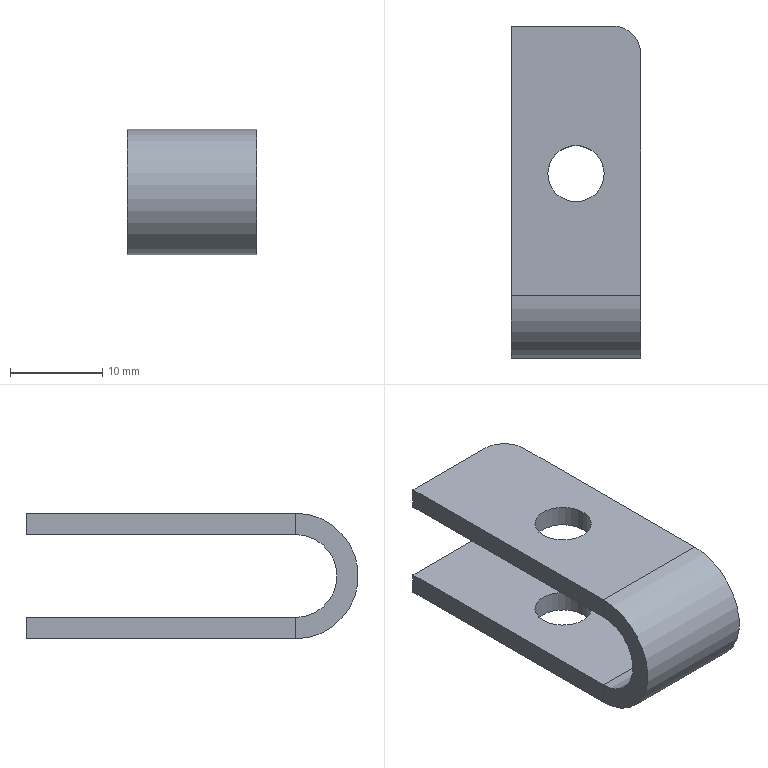Part | SolidWorks | features Fillet 1, FlatPattern 1, ICE 1, SMBaseFlange 1, SheetMetal 1 | 1 solid | 20 faces | box 14 x 36 x 13.6 mm | volume 2309 mm3 | plane 12 | cylinder 8 | commonest cylinder face diameters 6.1 x4 6 x2 9 x1 13.6 x1
STEP:
#1=CARTESIAN_POINT('',(3.95,13.2,4.5));
#2=VERTEX_POINT('',#1);
#3=CARTESIAN_POINT('',(10.05,13.2,4.5));
#4=VERTEX_POINT('',#3);
#5=CARTESIAN_POINT('',(7.,13.2,4.5));
#6=DIRECTION('',(0.,0.,1.));
#7=DIRECTION('',(0.,-1.,0.));
#8=AXIS2_PLACEMENT_3D('',#5,#6,#7);
#9=CIRCLE('',#8,3.05);
#10=EDGE_CURVE('',#2,#4,#9,.T.);
#11=ORIENTED_EDGE('',*,*,#10,.F.);
#12=CARTESIAN_POINT('',(3.95,13.2,6.8));
#13=VERTEX_POINT('',#12);
#14=CARTESIAN_POINT('',(3.95,13.2,-6.8));
#15=DIRECTION('',(0.,0.,1.));
#16=VECTOR('',#15,1000.);
#17=LINE('',#14,#16);
#18=EDGE_CURVE('',#2,#13,#17,.T.);
#19=ORIENTED_EDGE('',*,*,#18,.T.);
#20=CARTESIAN_POINT('',(10.05,13.2,6.8));
#21=VERTEX_POINT('',#20);
#22=CARTESIAN_POINT('',(7.,13.2,6.8));
#23=DIRECTION('',(0.,0.,1.));
#24=DIRECTION('',(1.,0.,0.));
#25=AXIS2_PLACEMENT_3D('',#22,#23,#24);
#26=CIRCLE('',#25,3.05);
#27=EDGE_CURVE('',#13,#21,#26,.T.);
#28=ORIENTED_EDGE('',*,*,#27,.T.);
#29=CARTESIAN_POINT('',(10.05,13.2,-6.8));
#30=DIRECTION('',(0.,0.,1.));
#31=VECTOR('',#30,1000.);
#32=LINE('',#29,#31);
#33=EDGE_CURVE('',#4,#21,#32,.T.);
#34=ORIENTED_EDGE('',*,*,#33,.F.);
#35=EDGE_LOOP('',(#11,#19,#28,#34));
#36=FACE_OUTER_BOUND('',#35,.T.);
#37=CARTESIAN_POINT('',(7.,13.2,-6.8));
#38=DIRECTION('',(0.,0.,1.));
#39=DIRECTION('',(1.,0.,0.));
#40=AXIS2_PLACEMENT_3D('',#37,#38,#39);
#41=CYLINDRICAL_SURFACE('',#40,3.05);
#42=ADVANCED_FACE('',(#36),#41,.F.);
#43=CARTESIAN_POINT('',(3.95,13.2,-6.8));
#44=VERTEX_POINT('',#43);
#45=CARTESIAN_POINT('',(10.05,13.2,-6.8));
#46=VERTEX_POINT('',#45);
#47=CARTESIAN_POINT('',(7.,13.2,-6.8));
#48=DIRECTION('',(0.,0.,1.));
#49=DIRECTION('',(1.,0.,0.));
#50=AXIS2_PLACEMENT_3D('',#47,#48,#49);
#51=CIRCLE('',#50,3.05);
#52=EDGE_CURVE('',#44,#46,#51,.T.);
#53=ORIENTED_EDGE('',*,*,#52,.F.);
#54=CARTESIAN_POINT('',(3.95,13.2,-4.5));
#55=VERTEX_POINT('',#54);
#56=CARTESIAN_POINT('',(3.95,13.2,-6.8));
#57=DIRECTION('',(0.,0.,1.));
#58=VECTOR('',#57,1000.);
#59=LINE('',#56,#58);
#60=EDGE_CURVE('',#44,#55,#59,.T.);
#61=ORIENTED_EDGE('',*,*,#60,.T.);
#62=CARTESIAN_POINT('',(10.05,13.2,-4.5));
#63=VERTEX_POINT('',#62);
#64=CARTESIAN_POINT('',(7.,13.2,-4.5));
#65=DIRECTION('',(0.,0.,-1.));
#66=DIRECTION('',(0.,1.,0.));
#67=AXIS2_PLACEMENT_3D('',#64,#65,#66);
#68=CIRCLE('',#67,3.05);
#69=EDGE_CURVE('',#63,#55,#68,.T.);
#70=ORIENTED_EDGE('',*,*,#69,.F.);
#71=CARTESIAN_POINT('',(10.05,13.2,-6.8));
#72=DIRECTION('',(0.,0.,1.));
#73=VECTOR('',#72,1000.);
#74=LINE('',#71,#73);
#75=EDGE_CURVE('',#46,#63,#74,.T.);
#76=ORIENTED_EDGE('',*,*,#75,.F.);
#77=EDGE_LOOP('',(#53,#61,#70,#76));
#78=FACE_OUTER_BOUND('',#77,.T.);
#79=CARTESIAN_POINT('',(7.,13.2,-6.8));
#80=DIRECTION('',(0.,0.,1.));
#81=DIRECTION('',(1.,0.,0.));
#82=AXIS2_PLACEMENT_3D('',#79,#80,#81);
#83=CYLINDRICAL_SURFACE('',#82,3.05);
#84=ADVANCED_FACE('',(#78),#83,.F.);
#85=CARTESIAN_POINT('',(14.,0.,6.8));
#86=VERTEX_POINT('',#85);
#87=CARTESIAN_POINT('',(14.,0.,4.5));
#88=VERTEX_POINT('',#87);
#89=CARTESIAN_POINT('',(14.,0.,6.8));
#90=DIRECTION('',(0.,0.,-1.));
#91=VECTOR('',#90,1000.);
#92=LINE('',#89,#91);
#93=EDGE_CURVE('',#86,#88,#92,.T.);
#94=ORIENTED_EDGE('',*,*,#93,.F.);
#95=CARTESIAN_POINT('',(14.,0.,-6.8));
#96=VERTEX_POINT('',#95);
#97=CARTESIAN_POINT('',(14.,0.,0.));
#98=DIRECTION('',(-1.,0.,0.));
#99=DIRECTION('',(0.,0.,-1.));
#100=AXIS2_PLACEMENT_3D('',#97,#98,#99);
#101=CIRCLE('',#100,6.8);
#102=EDGE_CURVE('',#96,#86,#101,.T.);
#103=ORIENTED_EDGE('',*,*,#102,.F.);
#104=CARTESIAN_POINT('',(14.,0.,-4.5));
#105=VERTEX_POINT('',#104);
#106=CARTESIAN_POINT('',(14.,0.,-4.5));
#107=DIRECTION('',(0.,0.,-1.));
#108=VECTOR('',#107,1000.);
#109=LINE('',#106,#108);
#110=EDGE_CURVE('',#105,#96,#109,.T.);
#111=ORIENTED_EDGE('',*,*,#110,.F.);
#112=CARTESIAN_POINT('',(14.,0.,0.));
#113=DIRECTION('',(-1.,0.,0.));
#114=DIRECTION('',(0.,0.,-1.));
#115=AXIS2_PLACEMENT_3D('',#112,#113,#114);
#116=CIRCLE('',#115,4.5);
#117=EDGE_CURVE('',#105,#88,#116,.T.);
#118=ORIENTED_EDGE('',*,*,#117,.T.);
#119=EDGE_LOOP('',(#94,#103,#111,#118));
#120=FACE_OUTER_BOUND('',#119,.T.);
#121=CARTESIAN_POINT('',(14.,0.,6.8));
#122=DIRECTION('',(1.,0.,0.));
#123=DIRECTION('',(0.,0.,-1.));
#124=AXIS2_PLACEMENT_3D('',#121,#122,#123);
#125=PLANE('',#124);
#126=ADVANCED_FACE('',(#120),#125,.T.);
#127=CARTESIAN_POINT('',(14.,26.2,4.5));
#128=VERTEX_POINT('',#127);
#129=CARTESIAN_POINT('',(14.,0.,4.5));
#130=DIRECTION('',(0.,1.,0.));
#131=VECTOR('',#130,1000.);
#132=LINE('',#129,#131);
#133=EDGE_CURVE('',#88,#128,#132,.T.);
#134=ORIENTED_EDGE('',*,*,#133,.T.);
#135=CARTESIAN_POINT('',(14.,26.2,6.8));
#136=VERTEX_POINT('',#135);
#137=CARTESIAN_POINT('',(14.,26.2,-4.5));
#138=DIRECTION('',(0.,0.,1.));
#139=VECTOR('',#138,1000.);
#140=LINE('',#137,#139);
#141=EDGE_CURVE('',#128,#136,#140,.T.);
#142=ORIENTED_EDGE('',*,*,#141,.T.);
#143=CARTESIAN_POINT('',(14.,0.,6.8));
#144=DIRECTION('',(0.,1.,0.));
#145=VECTOR('',#144,1000.);
#146=LINE('',#143,#145);
#147=EDGE_CURVE('',#86,#136,#146,.T.);
#148=ORIENTED_EDGE('',*,*,#147,.F.);
#149=ORIENTED_EDGE('',*,*,#93,.T.);
#150=EDGE_LOOP('',(#134,#142,#148,#149));
#151=FACE_OUTER_BOUND('',#150,.T.);
#152=CARTESIAN_POINT('',(14.,0.,-4.5));
#153=DIRECTION('',(1.,0.,0.));
#154=DIRECTION('',(0.,0.,-1.));
#155=AXIS2_PLACEMENT_3D('',#152,#153,#154);
#156=PLANE('',#155);
#157=ADVANCED_FACE('',(#151),#156,.T.);
#158=CARTESIAN_POINT('',(0.,0.,-6.8));
#159=VERTEX_POINT('',#158);
#160=CARTESIAN_POINT('',(0.,0.,-4.5));
#161=VERTEX_POINT('',#160);
#162=CARTESIAN_POINT('',(0.,0.,-6.8));
#163=DIRECTION('',(0.,0.,1.));
#164=VECTOR('',#163,1000.);
#165=LINE('',#162,#164);
#166=EDGE_CURVE('',#159,#161,#165,.T.);
#167=ORIENTED_EDGE('',*,*,#166,.F.);
#168=CARTESIAN_POINT('',(0.,0.,6.8));
#169=VERTEX_POINT('',#168);
#170=CARTESIAN_POINT('',(0.,0.,0.));
#171=DIRECTION('',(-1.,0.,0.));
#172=DIRECTION('',(0.,0.,-1.));
#173=AXIS2_PLACEMENT_3D('',#170,#171,#172);
#174=CIRCLE('',#173,6.8);
#175=EDGE_CURVE('',#159,#169,#174,.T.);
#176=ORIENTED_EDGE('',*,*,#175,.T.);
#177=CARTESIAN_POINT('',(0.,0.,4.5));
#178=VERTEX_POINT('',#177);
#179=CARTESIAN_POINT('',(0.,0.,4.5));
#180=DIRECTION('',(0.,0.,1.));
#181=VECTOR('',#180,1000.);
#182=LINE('',#179,#181);
#183=EDGE_CURVE('',#178,#169,#182,.T.);
#184=ORIENTED_EDGE('',*,*,#183,.F.);
#185=CARTESIAN_POINT('',(0.,0.,0.));
#186=DIRECTION('',(-1.,0.,0.));
#187=DIRECTION('',(0.,0.,-1.));
#188=AXIS2_PLACEMENT_3D('',#185,#186,#187);
#189=CIRCLE('',#188,4.5);
#190=EDGE_CURVE('',#161,#178,#189,.T.);
#191=ORIENTED_EDGE('',*,*,#190,.F.);
#192=EDGE_LOOP('',(#167,#176,#184,#191));
#193=FACE_OUTER_BOUND('',#192,.T.);
#194=CARTESIAN_POINT('',(0.,0.,-6.8));
#195=DIRECTION('',(-1.,0.,0.));
#196=DIRECTION('',(0.,0.,1.));
#197=AXIS2_PLACEMENT_3D('',#194,#195,#196);
#198=PLANE('',#197);
#199=ADVANCED_FACE('',(#193),#198,.T.);
#200=CARTESIAN_POINT('',(0.,29.2,-6.8));
#201=VERTEX_POINT('',#200);
#202=CARTESIAN_POINT('',(0.,29.2,-6.8));
#203=DIRECTION('',(0.,-1.,0.));
#204=VECTOR('',#203,1000.);
#205=LINE('',#202,#204);
#206=EDGE_CURVE('',#201,#159,#205,.T.);
#207=ORIENTED_EDGE('',*,*,#206,.T.);
#208=ORIENTED_EDGE('',*,*,#166,.T.);
#209=CARTESIAN_POINT('',(0.,29.2,-4.5));
#210=VERTEX_POINT('',#209);
#211=CARTESIAN_POINT('',(0.,29.2,-4.5));
#212=DIRECTION('',(0.,-1.,0.));
#213=VECTOR('',#212,1000.);
#214=LINE('',#211,#213);
#215=EDGE_CURVE('',#210,#161,#214,.T.);
#216=ORIENTED_EDGE('',*,*,#215,.F.);
#217=CARTESIAN_POINT('',(0.,29.2,-4.5));
#218=DIRECTION('',(0.,0.,-1.));
#219=VECTOR('',#218,1000.);
#220=LINE('',#217,#219);
#221=EDGE_CURVE('',#210,#201,#220,.T.);
#222=ORIENTED_EDGE('',*,*,#221,.T.);
#223=EDGE_LOOP('',(#207,#208,#216,#222));
#224=FACE_OUTER_BOUND('',#223,.T.);
#225=CARTESIAN_POINT('',(0.,0.,4.5));
#226=DIRECTION('',(-1.,0.,0.));
#227=DIRECTION('',(0.,0.,1.));
#228=AXIS2_PLACEMENT_3D('',#225,#226,#227);
#229=PLANE('',#228);
#230=ADVANCED_FACE('',(#224),#229,.T.);
#231=CARTESIAN_POINT('',(7.,13.2,4.5));
#232=DIRECTION('',(0.,0.,1.));
#233=DIRECTION('',(0.,-1.,0.));
#234=AXIS2_PLACEMENT_3D('',#231,#232,#233);
#235=CIRCLE('',#234,3.05);
#236=EDGE_CURVE('',#4,#2,#235,.T.);
#237=ORIENTED_EDGE('',*,*,#236,.T.);
#238=ORIENTED_EDGE('',*,*,#10,.T.);
#239=EDGE_LOOP('',(#237,#238));
#240=FACE_BOUND('',#239,.T.);
#241=CARTESIAN_POINT('',(11.,29.2,4.5));
#242=VERTEX_POINT('',#241);
#243=CARTESIAN_POINT('',(0.,29.2,4.5));
#244=VERTEX_POINT('',#243);
#245=CARTESIAN_POINT('',(14.,29.2,4.5));
#246=DIRECTION('',(-1.,0.,0.));
#247=VECTOR('',#246,1000.);
#248=LINE('',#245,#247);
#249=EDGE_CURVE('',#242,#244,#248,.T.);
#250=ORIENTED_EDGE('',*,*,#249,.F.);
#251=CARTESIAN_POINT('',(11.,26.2,4.5));
#252=DIRECTION('',(0.,0.,-1.));
#253=DIRECTION('',(0.,-1.,0.));
#254=AXIS2_PLACEMENT_3D('',#251,#252,#253);
#255=CIRCLE('',#254,3.);
#256=EDGE_CURVE('',#242,#128,#255,.T.);
#257=ORIENTED_EDGE('',*,*,#256,.T.);
#258=ORIENTED_EDGE('',*,*,#133,.F.);
#259=CARTESIAN_POINT('',(14.,0.,4.5));
#260=DIRECTION('',(-1.,0.,0.));
#261=VECTOR('',#260,1000.);
#262=LINE('',#259,#261);
#263=EDGE_CURVE('',#88,#178,#262,.T.);
#264=ORIENTED_EDGE('',*,*,#263,.T.);
#265=CARTESIAN_POINT('',(0.,0.,4.5));
#266=DIRECTION('',(0.,1.,0.));
#267=VECTOR('',#266,1000.);
#268=LINE('',#265,#267);
#269=EDGE_CURVE('',#178,#244,#268,.T.);
#270=ORIENTED_EDGE('',*,*,#269,.T.);
#271=EDGE_LOOP('',(#250,#257,#258,#264,#270));
#272=FACE_OUTER_BOUND('',#271,.T.);
#273=CARTESIAN_POINT('',(14.,0.,4.5));
#274=DIRECTION('',(0.,0.,1.));
#275=DIRECTION('',(0.,-1.,0.));
#276=AXIS2_PLACEMENT_3D('',#273,#274,#275);
#277=PLANE('',#276);
#278=ADVANCED_FACE('',(#240,#272),#277,.F.);
#279=CARTESIAN_POINT('',(11.,29.2,6.8));
#280=VERTEX_POINT('',#279);
#281=CARTESIAN_POINT('',(0.,29.2,6.8));
#282=VERTEX_POINT('',#281);
#283=CARTESIAN_POINT('',(14.,29.2,6.8));
#284=DIRECTION('',(-1.,0.,0.));
#285=VECTOR('',#284,1000.);
#286=LINE('',#283,#285);
#287=EDGE_CURVE('',#280,#282,#286,.T.);
#288=ORIENTED_EDGE('',*,*,#287,.F.);
#289=CARTESIAN_POINT('',(11.,29.2,6.8));
#290=DIRECTION('',(0.,0.,-1.));
#291=VECTOR('',#290,1000.);
#292=LINE('',#289,#291);
#293=EDGE_CURVE('',#280,#242,#292,.T.);
#294=ORIENTED_EDGE('',*,*,#293,.T.);
#295=ORIENTED_EDGE('',*,*,#249,.T.);
#296=CARTESIAN_POINT('',(0.,29.2,6.8));
#297=DIRECTION('',(0.,0.,-1.));
#298=VECTOR('',#297,1000.);
#299=LINE('',#296,#298);
#300=EDGE_CURVE('',#282,#244,#299,.T.);
#301=ORIENTED_EDGE('',*,*,#300,.F.);
#302=EDGE_LOOP('',(#288,#294,#295,#301));
#303=FACE_OUTER_BOUND('',#302,.T.);
#304=CARTESIAN_POINT('',(14.,29.2,6.8));
#305=DIRECTION('',(0.,1.,0.));
#306=DIRECTION('',(0.,0.,1.));
#307=AXIS2_PLACEMENT_3D('',#304,#305,#306);
#308=PLANE('',#307);
#309=ADVANCED_FACE('',(#303),#308,.T.);
#310=CARTESIAN_POINT('',(7.,13.2,6.8));
#311=DIRECTION('',(0.,0.,1.));
#312=DIRECTION('',(1.,0.,0.));
#313=AXIS2_PLACEMENT_3D('',#310,#311,#312);
#314=CIRCLE('',#313,3.05);
#315=EDGE_CURVE('',#21,#13,#314,.T.);
#316=ORIENTED_EDGE('',*,*,#315,.F.);
#317=ORIENTED_EDGE('',*,*,#27,.F.);
#318=EDGE_LOOP('',(#316,#317));
#319=FACE_BOUND('',#318,.T.);
#320=ORIENTED_EDGE('',*,*,#147,.T.);
#321=CARTESIAN_POINT('',(11.,26.2,6.8));
#322=DIRECTION('',(0.,0.,1.));
#323=DIRECTION('',(0.,-1.,0.));
#324=AXIS2_PLACEMENT_3D('',#321,#322,#323);
#325=CIRCLE('',#324,3.);
#326=EDGE_CURVE('',#136,#280,#325,.T.);
#327=ORIENTED_EDGE('',*,*,#326,.T.);
#328=ORIENTED_EDGE('',*,*,#287,.T.);
#329=CARTESIAN_POINT('',(0.,0.,6.8));
#330=DIRECTION('',(0.,1.,0.));
#331=VECTOR('',#330,1000.);
#332=LINE('',#329,#331);
#333=EDGE_CURVE('',#169,#282,#332,.T.);
#334=ORIENTED_EDGE('',*,*,#333,.F.);
#335=CARTESIAN_POINT('',(14.,0.,6.8));
#336=DIRECTION('',(-1.,0.,0.));
#337=VECTOR('',#336,1000.);
#338=LINE('',#335,#337);
#339=EDGE_CURVE('',#86,#169,#338,.T.);
#340=ORIENTED_EDGE('',*,*,#339,.F.);
#341=EDGE_LOOP('',(#320,#327,#328,#334,#340));
#342=FACE_OUTER_BOUND('',#341,.T.);
#343=CARTESIAN_POINT('',(14.,0.,6.8));
#344=DIRECTION('',(0.,0.,1.));
#345=DIRECTION('',(0.,-1.,0.));
#346=AXIS2_PLACEMENT_3D('',#343,#344,#345);
#347=PLANE('',#346);
#348=ADVANCED_FACE('',(#319,#342),#347,.T.);
#349=ORIENTED_EDGE('',*,*,#175,.F.);
#350=CARTESIAN_POINT('',(14.,0.,-6.8));
#351=DIRECTION('',(-1.,0.,0.));
#352=VECTOR('',#351,1000.);
#353=LINE('',#350,#352);
#354=EDGE_CURVE('',#96,#159,#353,.T.);
#355=ORIENTED_EDGE('',*,*,#354,.F.);
#356=ORIENTED_EDGE('',*,*,#102,.T.);
#357=ORIENTED_EDGE('',*,*,#339,.T.);
#358=EDGE_LOOP('',(#349,#355,#356,#357));
#359=FACE_OUTER_BOUND('',#358,.T.);
#360=CARTESIAN_POINT('',(14.,0.,0.));
#361=DIRECTION('',(-1.,0.,0.));
#362=DIRECTION('',(0.,0.,1.));
#363=AXIS2_PLACEMENT_3D('',#360,#361,#362);
#364=CYLINDRICAL_SURFACE('',#363,6.8);
#365=ADVANCED_FACE('',(#359),#364,.T.);
#366=CARTESIAN_POINT('',(7.,13.2,-6.8));
#367=DIRECTION('',(0.,0.,1.));
#368=DIRECTION('',(1.,0.,0.));
#369=AXIS2_PLACEMENT_3D('',#366,#367,#368);
#370=CIRCLE('',#369,3.05);
#371=EDGE_CURVE('',#46,#44,#370,.T.);
#372=ORIENTED_EDGE('',*,*,#371,.T.);
#373=ORIENTED_EDGE('',*,*,#52,.T.);
#374=EDGE_LOOP('',(#372,#373));
#375=FACE_BOUND('',#374,.T.);
#376=CARTESIAN_POINT('',(11.,29.2,-6.8));
#377=VERTEX_POINT('',#376);
#378=CARTESIAN_POINT('',(14.,29.2,-6.8));
#379=DIRECTION('',(-1.,0.,0.));
#380=VECTOR('',#379,1000.);
#381=LINE('',#378,#380);
#382=EDGE_CURVE('',#377,#201,#381,.T.);
#383=ORIENTED_EDGE('',*,*,#382,.F.);
#384=CARTESIAN_POINT('',(14.,26.2,-6.8));
#385=VERTEX_POINT('',#384);
#386=CARTESIAN_POINT('',(11.,26.2,-6.8));
#387=DIRECTION('',(0.,0.,-1.));
#388=DIRECTION('',(0.,1.,0.));
#389=AXIS2_PLACEMENT_3D('',#386,#387,#388);
#390=CIRCLE('',#389,3.);
#391=EDGE_CURVE('',#377,#385,#390,.T.);
#392=ORIENTED_EDGE('',*,*,#391,.T.);
#393=CARTESIAN_POINT('',(14.,29.2,-6.8));
#394=DIRECTION('',(0.,-1.,0.));
#395=VECTOR('',#394,1000.);
#396=LINE('',#393,#395);
#397=EDGE_CURVE('',#385,#96,#396,.T.);
#398=ORIENTED_EDGE('',*,*,#397,.T.);
#399=ORIENTED_EDGE('',*,*,#354,.T.);
#400=ORIENTED_EDGE('',*,*,#206,.F.);
#401=EDGE_LOOP('',(#383,#392,#398,#399,#400));
#402=FACE_OUTER_BOUND('',#401,.T.);
#403=CARTESIAN_POINT('',(14.,29.2,-6.8));
#404=DIRECTION('',(0.,0.,-1.));
#405=DIRECTION('',(0.,1.,0.));
#406=AXIS2_PLACEMENT_3D('',#403,#404,#405);
#407=PLANE('',#406);
#408=ADVANCED_FACE('',(#375,#402),#407,.T.);
#409=CARTESIAN_POINT('',(11.,29.2,-4.5));
#410=VERTEX_POINT('',#409);
#411=CARTESIAN_POINT('',(14.,29.2,-4.5));
#412=DIRECTION('',(-1.,0.,0.));
#413=VECTOR('',#412,1000.);
#414=LINE('',#411,#413);
#415=EDGE_CURVE('',#410,#210,#414,.T.);
#416=ORIENTED_EDGE('',*,*,#415,.F.);
#417=CARTESIAN_POINT('',(11.,29.2,-6.8));
#418=DIRECTION('',(0.,0.,-1.));
#419=VECTOR('',#418,1000.);
#420=LINE('',#417,#419);
#421=EDGE_CURVE('',#410,#377,#420,.T.);
#422=ORIENTED_EDGE('',*,*,#421,.T.);
#423=ORIENTED_EDGE('',*,*,#382,.T.);
#424=ORIENTED_EDGE('',*,*,#221,.F.);
#425=EDGE_LOOP('',(#416,#422,#423,#424));
#426=FACE_OUTER_BOUND('',#425,.T.);
#427=CARTESIAN_POINT('',(14.,29.2,-4.5));
#428=DIRECTION('',(0.,1.,0.));
#429=DIRECTION('',(0.,0.,1.));
#430=AXIS2_PLACEMENT_3D('',#427,#428,#429);
#431=PLANE('',#430);
#432=ADVANCED_FACE('',(#426),#431,.T.);
#433=ORIENTED_EDGE('',*,*,#69,.T.);
#434=CARTESIAN_POINT('',(7.,13.2,-4.5));
#435=DIRECTION('',(0.,0.,-1.));
#436=DIRECTION('',(0.,1.,0.));
#437=AXIS2_PLACEMENT_3D('',#434,#435,#436);
#438=CIRCLE('',#437,3.05);
#439=EDGE_CURVE('',#55,#63,#438,.T.);
#440=ORIENTED_EDGE('',*,*,#439,.T.);
#441=EDGE_LOOP('',(#433,#440));
#442=FACE_BOUND('',#441,.T.);
#443=CARTESIAN_POINT('',(14.,26.2,-4.5));
#444=VERTEX_POINT('',#443);
#445=CARTESIAN_POINT('',(14.,29.2,-4.5));
#446=DIRECTION('',(0.,-1.,0.));
#447=VECTOR('',#446,1000.);
#448=LINE('',#445,#447);
#449=EDGE_CURVE('',#444,#105,#448,.T.);
#450=ORIENTED_EDGE('',*,*,#449,.F.);
#451=CARTESIAN_POINT('',(11.,26.2,-4.5));
#452=DIRECTION('',(0.,0.,1.));
#453=DIRECTION('',(0.,1.,0.));
#454=AXIS2_PLACEMENT_3D('',#451,#452,#453);
#455=CIRCLE('',#454,3.);
#456=EDGE_CURVE('',#444,#410,#455,.T.);
#457=ORIENTED_EDGE('',*,*,#456,.T.);
#458=ORIENTED_EDGE('',*,*,#415,.T.);
#459=ORIENTED_EDGE('',*,*,#215,.T.);
#460=CARTESIAN_POINT('',(14.,0.,-4.5));
#461=DIRECTION('',(-1.,0.,0.));
#462=VECTOR('',#461,1000.);
#463=LINE('',#460,#462);
#464=EDGE_CURVE('',#105,#161,#463,.T.);
#465=ORIENTED_EDGE('',*,*,#464,.F.);
#466=EDGE_LOOP('',(#450,#457,#458,#459,#465));
#467=FACE_OUTER_BOUND('',#466,.T.);
#468=CARTESIAN_POINT('',(14.,29.2,-4.5));
#469=DIRECTION('',(0.,0.,-1.));
#470=DIRECTION('',(0.,1.,0.));
#471=AXIS2_PLACEMENT_3D('',#468,#469,#470);
#472=PLANE('',#471);
#473=ADVANCED_FACE('',(#442,#467),#472,.F.);
#474=ORIENTED_EDGE('',*,*,#190,.T.);
#475=ORIENTED_EDGE('',*,*,#263,.F.);
#476=ORIENTED_EDGE('',*,*,#117,.F.);
#477=ORIENTED_EDGE('',*,*,#464,.T.);
#478=EDGE_LOOP('',(#474,#475,#476,#477));
#479=FACE_OUTER_BOUND('',#478,.T.);
#480=CARTESIAN_POINT('',(14.,0.,0.));
#481=DIRECTION('',(-1.,0.,0.));
#482=DIRECTION('',(0.,0.,1.));
#483=AXIS2_PLACEMENT_3D('',#480,#481,#482);
#484=CYLINDRICAL_SURFACE('',#483,4.5);
#485=ADVANCED_FACE('',(#479),#484,.F.);
#486=ORIENTED_EDGE('',*,*,#397,.F.);
#487=CARTESIAN_POINT('',(14.,26.2,-4.5));
#488=DIRECTION('',(0.,0.,1.));
#489=VECTOR('',#488,1000.);
#490=LINE('',#487,#489);
#491=EDGE_CURVE('',#385,#444,#490,.T.);
#492=ORIENTED_EDGE('',*,*,#491,.T.);
#493=ORIENTED_EDGE('',*,*,#449,.T.);
#494=ORIENTED_EDGE('',*,*,#110,.T.);
#495=EDGE_LOOP('',(#486,#492,#493,#494));
#496=FACE_OUTER_BOUND('',#495,.T.);
#497=CARTESIAN_POINT('',(14.,0.,0.));
#498=DIRECTION('',(-1.,0.,0.));
#499=DIRECTION('',(0.,0.,1.));
#500=AXIS2_PLACEMENT_3D('',#497,#498,#499);
#501=PLANE('',#500);
#502=ADVANCED_FACE('',(#496),#501,.F.);
#503=ORIENTED_EDGE('',*,*,#269,.F.);
#504=ORIENTED_EDGE('',*,*,#183,.T.);
#505=ORIENTED_EDGE('',*,*,#333,.T.);
#506=ORIENTED_EDGE('',*,*,#300,.T.);
#507=EDGE_LOOP('',(#503,#504,#505,#506));
#508=FACE_OUTER_BOUND('',#507,.T.);
#509=CARTESIAN_POINT('',(0.,0.,0.));
#510=DIRECTION('',(-1.,0.,0.));
#511=DIRECTION('',(0.,0.,1.));
#512=AXIS2_PLACEMENT_3D('',#509,#510,#511);
#513=PLANE('',#512);
#514=ADVANCED_FACE('',(#508),#513,.T.);
#515=ORIENTED_EDGE('',*,*,#60,.F.);
#516=ORIENTED_EDGE('',*,*,#371,.F.);
#517=ORIENTED_EDGE('',*,*,#75,.T.);
#518=ORIENTED_EDGE('',*,*,#439,.F.);
#519=EDGE_LOOP('',(#515,#516,#517,#518));
#520=FACE_OUTER_BOUND('',#519,.T.);
#521=CARTESIAN_POINT('',(7.,13.2,-6.8));
#522=DIRECTION('',(0.,0.,1.));
#523=DIRECTION('',(1.,0.,0.));
#524=AXIS2_PLACEMENT_3D('',#521,#522,#523);
#525=CYLINDRICAL_SURFACE('',#524,3.05);
#526=ADVANCED_FACE('',(#520),#525,.F.);
#527=ORIENTED_EDGE('',*,*,#18,.F.);
#528=ORIENTED_EDGE('',*,*,#236,.F.);
#529=ORIENTED_EDGE('',*,*,#33,.T.);
#530=ORIENTED_EDGE('',*,*,#315,.T.);
#531=EDGE_LOOP('',(#527,#528,#529,#530));
#532=FACE_OUTER_BOUND('',#531,.T.);
#533=CARTESIAN_POINT('',(7.,13.2,-6.8));
#534=DIRECTION('',(0.,0.,1.));
#535=DIRECTION('',(1.,0.,0.));
#536=AXIS2_PLACEMENT_3D('',#533,#534,#535);
#537=CYLINDRICAL_SURFACE('',#536,3.05);
#538=ADVANCED_FACE('',(#532),#537,.F.);
#539=ORIENTED_EDGE('',*,*,#456,.F.);
#540=ORIENTED_EDGE('',*,*,#491,.F.);
#541=ORIENTED_EDGE('',*,*,#391,.F.);
#542=ORIENTED_EDGE('',*,*,#421,.F.);
#543=EDGE_LOOP('',(#539,#540,#541,#542));
#544=FACE_OUTER_BOUND('',#543,.T.);
#545=CARTESIAN_POINT('',(11.,26.2,-4.5));
#546=DIRECTION('',(0.,0.,1.));
#547=DIRECTION('',(1.,0.,0.));
#548=AXIS2_PLACEMENT_3D('',#545,#546,#547);
#549=CYLINDRICAL_SURFACE('',#548,3.);
#550=ADVANCED_FACE('',(#544),#549,.T.);
#551=ORIENTED_EDGE('',*,*,#326,.F.);
#552=ORIENTED_EDGE('',*,*,#141,.F.);
#553=ORIENTED_EDGE('',*,*,#256,.F.);
#554=ORIENTED_EDGE('',*,*,#293,.F.);
#555=EDGE_LOOP('',(#551,#552,#553,#554));
#556=FACE_OUTER_BOUND('',#555,.T.);
#557=CARTESIAN_POINT('',(11.,26.2,6.8));
#558=DIRECTION('',(0.,0.,-1.));
#559=DIRECTION('',(-1.,0.,0.));
#560=AXIS2_PLACEMENT_3D('',#557,#558,#559);
#561=CYLINDRICAL_SURFACE('',#560,3.);
#562=ADVANCED_FACE('',(#556),#561,.T.);
#563=CLOSED_SHELL('',(#42,#84,#126,#157,#199,#230,#278,#309,#348,#365,#408,#432,#473,#485,#502,#514,#526,#538,#550,#562));
#564=MANIFOLD_SOLID_BREP('',#563);
#565=CARTESIAN_POINT('',(0.,0.,0.));
#566=DIRECTION('',(0.,0.,1.));
#567=DIRECTION('',(1.,0.,0.));
#568=AXIS2_PLACEMENT_3D('',#565,#566,#567);
#569=(LENGTH_UNIT()NAMED_UNIT(*)SI_UNIT(.MILLI.,.METRE.));
#570=UNCERTAINTY_MEASURE_WITH_UNIT(LENGTH_MEASURE(0.00001),#569,'','');
#571=(NAMED_UNIT(*)PLANE_ANGLE_UNIT()SI_UNIT($,.RADIAN.));
#572=(NAMED_UNIT(*)SI_UNIT($,.STERADIAN.)SOLID_ANGLE_UNIT());
#573=(GEOMETRIC_REPRESENTATION_CONTEXT(3)GLOBAL_UNCERTAINTY_ASSIGNED_CONTEXT((#570))GLOBAL_UNIT_ASSIGNED_CONTEXT((#569,#571,#572))REPRESENTATION_CONTEXT('',''));
#574=ADVANCED_BREP_SHAPE_REPRESENTATION('',(#564,#568),#573);